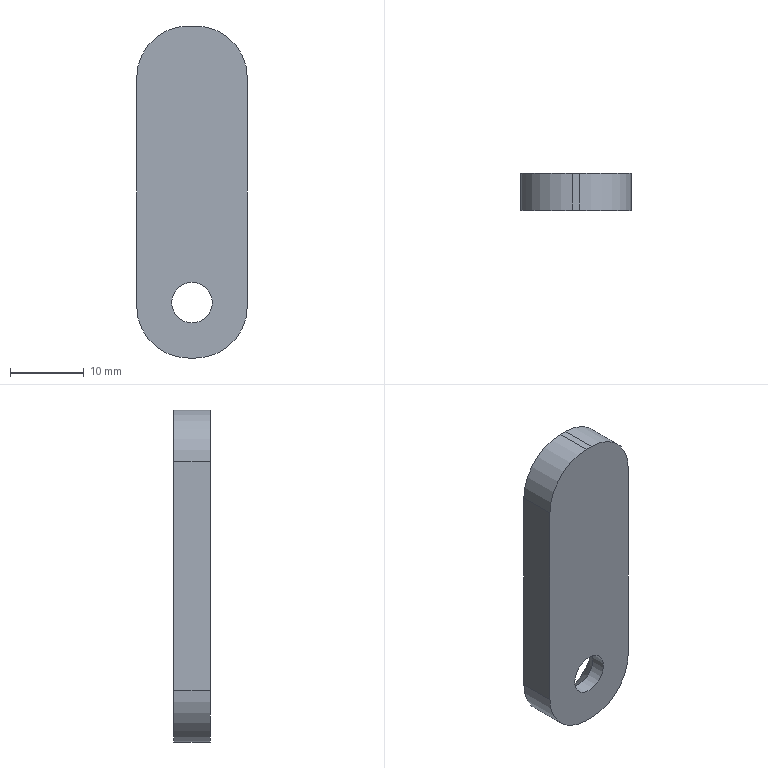Part | STEP file | solid 58 | 1 solid | 12 faces | box 15 x 5 x 45 mm | volume 2940 mm3 | plane 6 | cylinder 5 | cone 1 | commonest cylinder face diameters 14 x4 5.5 x1